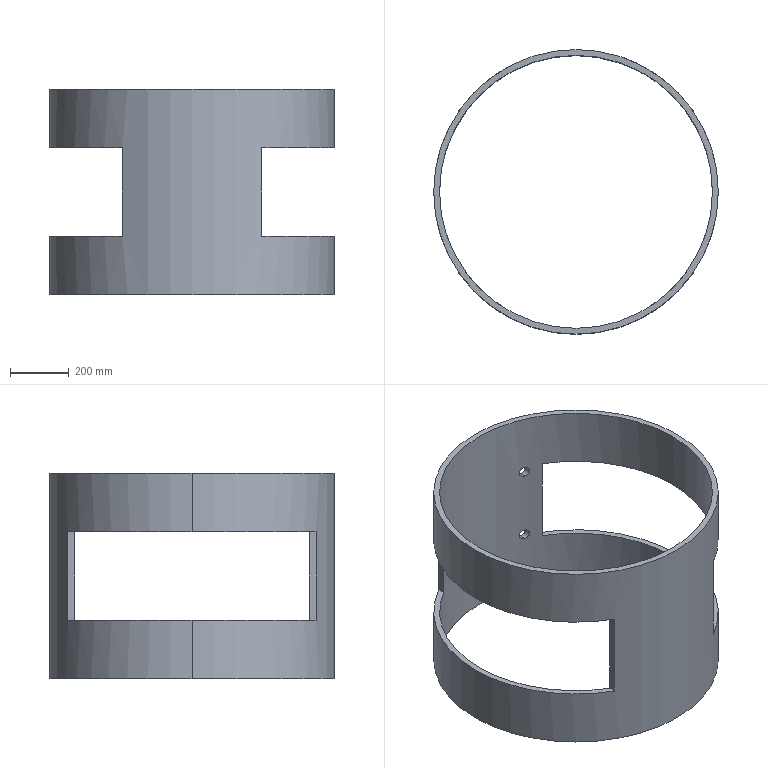Part | SolidWorks | features ICE 2, Extrusion 1 | 1 solid | 18 faces | box 970 x 970 x 700 mm | volume 29802772 mm3 | plane 10 | cylinder 8 | commonest cylinder face diameters 35 x4 930 x2 970 x2
STEP:
#1=CARTESIAN_POINT('',(180.,450.361,202.5));
#2=VERTEX_POINT('',#1);
#3=CARTESIAN_POINT('',(180.,450.361,237.5));
#4=VERTEX_POINT('',#3);
#5=CARTESIAN_POINT('',(180.,450.361,202.5));
#6=CARTESIAN_POINT('',(178.89,450.805,202.5));
#7=CARTESIAN_POINT('',(177.794,451.238,202.605));
#8=CARTESIAN_POINT('',(176.172,451.872,202.915));
#9=CARTESIAN_POINT('',(175.635,452.081,203.044));
#10=CARTESIAN_POINT('',(174.569,452.494,203.355));
#11=CARTESIAN_POINT('',(174.037,452.699,203.538));
#12=CARTESIAN_POINT('',(172.473,453.298,204.162));
#13=CARTESIAN_POINT('',(171.479,453.675,204.674));
#14=CARTESIAN_POINT('',(170.061,454.208,205.585));
#15=CARTESIAN_POINT('',(169.601,454.38,205.914));
#16=CARTESIAN_POINT('',(168.706,454.713,206.62));
#17=CARTESIAN_POINT('',(168.27,454.874,207.001));
#18=CARTESIAN_POINT('',(167.03,455.332,208.196));
#19=CARTESIAN_POINT('',(166.286,455.604,209.068));
#20=CARTESIAN_POINT('',(165.296,455.963,210.493));
#21=CARTESIAN_POINT('',(164.988,456.075,210.987));
#22=CARTESIAN_POINT('',(164.416,456.281,212.016));
#23=CARTESIAN_POINT('',(164.156,456.375,212.545));
#24=CARTESIAN_POINT('',(163.462,456.624,214.16));
#25=CARTESIAN_POINT('',(163.108,456.75,215.277));
#26=CARTESIAN_POINT('',(162.746,456.879,217.019));
#27=CARTESIAN_POINT('',(162.653,456.912,217.612));
#28=CARTESIAN_POINT('',(162.532,456.956,218.794));
#29=CARTESIAN_POINT('',(162.47,456.977,219.975));
#30=CARTESIAN_POINT('',(162.528,456.957,221.155));
#31=CARTESIAN_POINT('',(162.646,456.915,222.335));
#32=CARTESIAN_POINT('',(162.737,456.883,222.928));
#33=CARTESIAN_POINT('',(163.094,456.755,224.675));
#34=CARTESIAN_POINT('',(163.446,456.63,225.796));
#35=CARTESIAN_POINT('',(164.138,456.381,227.416));
#36=CARTESIAN_POINT('',(164.398,456.288,227.948));
#37=CARTESIAN_POINT('',(164.966,456.082,228.977));
#38=CARTESIAN_POINT('',(165.274,455.971,229.472));
#39=CARTESIAN_POINT('',(166.262,455.612,230.902));
#40=CARTESIAN_POINT('',(167.008,455.339,231.781));
#41=CARTESIAN_POINT('',(168.672,454.726,233.389));
#42=CARTESIAN_POINT('',(169.564,454.394,234.093));
#43=CARTESIAN_POINT('',(170.986,453.86,235.01));
#44=CARTESIAN_POINT('',(171.474,453.676,235.293));
#45=CARTESIAN_POINT('',(172.477,453.296,235.811));
#46=CARTESIAN_POINT('',(172.993,453.099,236.046));
#47=CARTESIAN_POINT('',(174.55,452.502,236.667));
#48=CARTESIAN_POINT('',(175.613,452.091,236.977));
#49=CARTESIAN_POINT('',(177.244,451.453,237.29));
#50=CARTESIAN_POINT('',(177.795,451.236,237.369));
#51=CARTESIAN_POINT('',(178.9,450.799,237.474));
#52=CARTESIAN_POINT('',(179.451,450.58,237.5));
#53=CARTESIAN_POINT('',(180.,450.361,237.5));
#54=B_SPLINE_CURVE_WITH_KNOTS('',3,(#5,#6,#7,#8,#9,#10,#11,#12,#13,#14,#15,#16,#17,#18,#19,#20,#21,#22,#23,#24,#25,#26,#27,#28,#29,#30,#31,#32,#33,#34,#35,#36,#37,#38,#39,#40,#41,#42,#43,#44,#45,#46,#47,#48,#49,#50,#51,#52,#53),.UNSPECIFIED.,.F.,.F.,(4,2,2,2,2,2,2,2,2,2,2,2,1,2,2,2,2,2,2,2,2,2,2,2,4),(0.,0.003538,0.005306,0.007075,0.01061,0.01238,0.01415,0.01769,0.01946,0.02123,0.02476,0.02653,0.0283,0.03007,0.03184,0.03538,0.03714,0.03891,0.04245,0.04599,0.04776,0.04953,0.05306,0.05483,0.0566),.UNSPECIFIED.);
#55=EDGE_CURVE('',#2,#4,#54,.T.);
#56=ORIENTED_EDGE('',*,*,#55,.T.);
#57=CARTESIAN_POINT('',(180.,428.748,237.5));
#58=VERTEX_POINT('',#57);
#59=CARTESIAN_POINT('',(180.,700.,237.5));
#60=DIRECTION('',(0.,-1.,0.));
#61=VECTOR('',#60,1000.);
#62=LINE('',#59,#61);
#63=EDGE_CURVE('',#4,#58,#62,.T.);
#64=ORIENTED_EDGE('',*,*,#63,.T.);
#65=CARTESIAN_POINT('',(180.,428.748,202.5));
#66=VERTEX_POINT('',#65);
#67=CARTESIAN_POINT('',(180.,428.748,202.5));
#68=CARTESIAN_POINT('',(178.894,429.213,202.5));
#69=CARTESIAN_POINT('',(177.802,429.666,202.604));
#70=CARTESIAN_POINT('',(176.186,430.33,202.912));
#71=CARTESIAN_POINT('',(175.65,430.549,203.04));
#72=CARTESIAN_POINT('',(174.587,430.981,203.349));
#73=CARTESIAN_POINT('',(174.057,431.196,203.531));
#74=CARTESIAN_POINT('',(172.495,431.824,204.151));
#75=CARTESIAN_POINT('',(171.502,432.219,204.661));
#76=CARTESIAN_POINT('',(170.085,432.778,205.569));
#77=CARTESIAN_POINT('',(169.625,432.958,205.896));
#78=CARTESIAN_POINT('',(168.73,433.307,206.6));
#79=CARTESIAN_POINT('',(168.294,433.477,206.979));
#80=CARTESIAN_POINT('',(167.05,433.958,208.173));
#81=CARTESIAN_POINT('',(166.304,434.245,209.045));
#82=CARTESIAN_POINT('',(165.312,434.623,210.468));
#83=CARTESIAN_POINT('',(165.003,434.74,210.962));
#84=CARTESIAN_POINT('',(164.573,434.903,211.733));
#85=CARTESIAN_POINT('',(164.435,434.955,211.996));
#86=CARTESIAN_POINT('',(164.174,435.054,212.525));
#87=CARTESIAN_POINT('',(164.051,435.1,212.792));
#88=CARTESIAN_POINT('',(163.468,435.32,214.14));
#89=CARTESIAN_POINT('',(163.112,435.453,215.261));
#90=CARTESIAN_POINT('',(162.748,435.589,217.005));
#91=CARTESIAN_POINT('',(162.655,435.624,217.601));
#92=CARTESIAN_POINT('',(162.532,435.67,218.787));
#93=CARTESIAN_POINT('',(162.501,435.682,219.38));
#94=CARTESIAN_POINT('',(162.499,435.682,220.565));
#95=CARTESIAN_POINT('',(162.528,435.671,221.157));
#96=CARTESIAN_POINT('',(162.617,435.638,222.044));
#97=CARTESIAN_POINT('',(162.655,435.624,222.34));
#98=CARTESIAN_POINT('',(162.745,435.591,222.931));
#99=CARTESIAN_POINT('',(162.798,435.571,223.227));
#100=CARTESIAN_POINT('',(163.098,435.459,224.688));
#101=CARTESIAN_POINT('',(163.452,435.326,225.813));
#102=CARTESIAN_POINT('',(164.147,435.064,227.435));
#103=CARTESIAN_POINT('',(164.408,434.966,227.967));
#104=CARTESIAN_POINT('',(164.979,434.749,228.998));
#105=CARTESIAN_POINT('',(165.288,434.632,229.494));
#106=CARTESIAN_POINT('',(166.279,434.254,230.924));
#107=CARTESIAN_POINT('',(167.028,433.967,231.803));
#108=CARTESIAN_POINT('',(168.694,433.322,233.407));
#109=CARTESIAN_POINT('',(169.587,432.974,234.11));
#110=CARTESIAN_POINT('',(171.008,432.414,235.024));
#111=CARTESIAN_POINT('',(171.496,432.22,235.305));
#112=CARTESIAN_POINT('',(172.498,431.821,235.821));
#113=CARTESIAN_POINT('',(173.013,431.615,236.054));
#114=CARTESIAN_POINT('',(174.567,430.99,236.673));
#115=CARTESIAN_POINT('',(175.628,430.559,236.981));
#116=CARTESIAN_POINT('',(177.253,429.891,237.292));
#117=CARTESIAN_POINT('',(177.803,429.664,237.37));
#118=CARTESIAN_POINT('',(178.904,429.207,237.474));
#119=CARTESIAN_POINT('',(179.453,428.978,237.5));
#120=CARTESIAN_POINT('',(180.,428.748,237.5));
#121=B_SPLINE_CURVE_WITH_KNOTS('',3,(#67,#68,#69,#70,#71,#72,#73,#74,#75,#76,#77,#78,#79,#80,#81,#82,#83,#84,#85,#86,#87,#88,#89,#90,#91,#92,#93,#94,#95,#96,#97,#98,#99,#100,#101,#102,#103,#104,#105,#106,#107,#108,#109,#110,#111,#112,#113,#114,#115,#116,#117,#118,#119,#120),.UNSPECIFIED.,.F.,.F.,(4,2,2,2,2,2,2,2,2,2,2,2,2,2,2,2,2,2,2,2,2,2,2,2,2,2,4),(0.,0.003549,0.005324,0.007098,0.01065,0.01242,0.0142,0.01775,0.01952,0.02041,0.0213,0.02484,0.02662,0.02839,0.03017,0.03106,0.03194,0.03549,0.03727,0.03904,0.04259,0.04614,0.04791,0.04969,0.05324,0.05501,0.05679),.UNSPECIFIED.);
#122=EDGE_CURVE('',#66,#58,#121,.T.);
#123=ORIENTED_EDGE('',*,*,#122,.F.);
#124=CARTESIAN_POINT('',(180.,700.,202.5));
#125=DIRECTION('',(0.,-1.,0.));
#126=VECTOR('',#125,1000.);
#127=LINE('',#124,#126);
#128=EDGE_CURVE('',#2,#66,#127,.T.);
#129=ORIENTED_EDGE('',*,*,#128,.F.);
#130=EDGE_LOOP('',(#56,#64,#123,#129));
#131=FACE_OUTER_BOUND('',#130,.T.);
#132=CARTESIAN_POINT('',(180.,700.,220.));
#133=DIRECTION('',(0.,-1.,0.));
#134=DIRECTION('',(0.,0.,-1.));
#135=AXIS2_PLACEMENT_3D('',#132,#133,#134);
#136=CYLINDRICAL_SURFACE('',#135,17.5);
#137=ADVANCED_FACE('',(#131),#136,.F.);
#138=CARTESIAN_POINT('',(180.,450.361,462.5));
#139=VERTEX_POINT('',#138);
#140=CARTESIAN_POINT('',(180.,450.361,497.5));
#141=VERTEX_POINT('',#140);
#142=CARTESIAN_POINT('',(180.,450.361,462.5));
#143=CARTESIAN_POINT('',(178.89,450.805,462.5));
#144=CARTESIAN_POINT('',(177.794,451.238,462.605));
#145=CARTESIAN_POINT('',(176.172,451.872,462.915));
#146=CARTESIAN_POINT('',(175.635,452.081,463.044));
#147=CARTESIAN_POINT('',(174.569,452.494,463.355));
#148=CARTESIAN_POINT('',(174.037,452.699,463.538));
#149=CARTESIAN_POINT('',(172.473,453.298,464.162));
#150=CARTESIAN_POINT('',(171.479,453.675,464.674));
#151=CARTESIAN_POINT('',(170.061,454.208,465.585));
#152=CARTESIAN_POINT('',(169.601,454.38,465.914));
#153=CARTESIAN_POINT('',(168.706,454.713,466.62));
#154=CARTESIAN_POINT('',(168.27,454.874,467.001));
#155=CARTESIAN_POINT('',(167.03,455.332,468.196));
#156=CARTESIAN_POINT('',(166.286,455.604,469.068));
#157=CARTESIAN_POINT('',(165.296,455.963,470.493));
#158=CARTESIAN_POINT('',(164.988,456.075,470.987));
#159=CARTESIAN_POINT('',(164.416,456.281,472.016));
#160=CARTESIAN_POINT('',(164.156,456.375,472.545));
#161=CARTESIAN_POINT('',(163.462,456.624,474.16));
#162=CARTESIAN_POINT('',(163.108,456.75,475.277));
#163=CARTESIAN_POINT('',(162.746,456.879,477.019));
#164=CARTESIAN_POINT('',(162.653,456.912,477.612));
#165=CARTESIAN_POINT('',(162.532,456.956,478.794));
#166=CARTESIAN_POINT('',(162.47,456.977,479.975));
#167=CARTESIAN_POINT('',(162.528,456.957,481.155));
#168=CARTESIAN_POINT('',(162.646,456.915,482.335));
#169=CARTESIAN_POINT('',(162.737,456.883,482.928));
#170=CARTESIAN_POINT('',(163.094,456.755,484.675));
#171=CARTESIAN_POINT('',(163.446,456.63,485.796));
#172=CARTESIAN_POINT('',(164.138,456.381,487.416));
#173=CARTESIAN_POINT('',(164.398,456.288,487.948));
#174=CARTESIAN_POINT('',(164.966,456.082,488.977));
#175=CARTESIAN_POINT('',(165.274,455.971,489.472));
#176=CARTESIAN_POINT('',(166.262,455.612,490.902));
#177=CARTESIAN_POINT('',(167.008,455.339,491.781));
#178=CARTESIAN_POINT('',(168.672,454.726,493.389));
#179=CARTESIAN_POINT('',(169.564,454.394,494.093));
#180=CARTESIAN_POINT('',(170.986,453.86,495.01));
#181=CARTESIAN_POINT('',(171.474,453.676,495.293));
#182=CARTESIAN_POINT('',(172.477,453.296,495.811));
#183=CARTESIAN_POINT('',(172.993,453.099,496.046));
#184=CARTESIAN_POINT('',(174.55,452.502,496.667));
#185=CARTESIAN_POINT('',(175.613,452.091,496.977));
#186=CARTESIAN_POINT('',(177.244,451.453,497.29));
#187=CARTESIAN_POINT('',(177.795,451.236,497.369));
#188=CARTESIAN_POINT('',(178.9,450.799,497.474));
#189=CARTESIAN_POINT('',(179.451,450.58,497.5));
#190=CARTESIAN_POINT('',(180.,450.361,497.5));
#191=B_SPLINE_CURVE_WITH_KNOTS('',3,(#142,#143,#144,#145,#146,#147,#148,#149,#150,#151,#152,#153,#154,#155,#156,#157,#158,#159,#160,#161,#162,#163,#164,#165,#166,#167,#168,#169,#170,#171,#172,#173,#174,#175,#176,#177,#178,#179,#180,#181,#182,#183,#184,#185,#186,#187,#188,#189,#190),.UNSPECIFIED.,.F.,.F.,(4,2,2,2,2,2,2,2,2,2,2,2,1,2,2,2,2,2,2,2,2,2,2,2,4),(0.,0.003538,0.005306,0.007075,0.01061,0.01238,0.01415,0.01769,0.01946,0.02123,0.02476,0.02653,0.0283,0.03007,0.03184,0.03538,0.03714,0.03891,0.04245,0.04599,0.04776,0.04953,0.05306,0.05483,0.0566),.UNSPECIFIED.);
#192=EDGE_CURVE('',#139,#141,#191,.T.);
#193=ORIENTED_EDGE('',*,*,#192,.T.);
#194=CARTESIAN_POINT('',(180.,428.748,497.5));
#195=VERTEX_POINT('',#194);
#196=CARTESIAN_POINT('',(180.,700.,497.5));
#197=DIRECTION('',(0.,-1.,0.));
#198=VECTOR('',#197,1000.);
#199=LINE('',#196,#198);
#200=EDGE_CURVE('',#141,#195,#199,.T.);
#201=ORIENTED_EDGE('',*,*,#200,.T.);
#202=CARTESIAN_POINT('',(180.,428.748,462.5));
#203=VERTEX_POINT('',#202);
#204=CARTESIAN_POINT('',(180.,428.748,462.5));
#205=CARTESIAN_POINT('',(178.894,429.213,462.5));
#206=CARTESIAN_POINT('',(177.802,429.666,462.604));
#207=CARTESIAN_POINT('',(176.186,430.33,462.912));
#208=CARTESIAN_POINT('',(175.65,430.549,463.04));
#209=CARTESIAN_POINT('',(174.587,430.981,463.349));
#210=CARTESIAN_POINT('',(174.057,431.196,463.531));
#211=CARTESIAN_POINT('',(172.495,431.824,464.151));
#212=CARTESIAN_POINT('',(171.502,432.219,464.661));
#213=CARTESIAN_POINT('',(170.085,432.778,465.569));
#214=CARTESIAN_POINT('',(169.625,432.958,465.896));
#215=CARTESIAN_POINT('',(168.73,433.307,466.6));
#216=CARTESIAN_POINT('',(168.294,433.477,466.979));
#217=CARTESIAN_POINT('',(167.05,433.958,468.173));
#218=CARTESIAN_POINT('',(166.304,434.245,469.045));
#219=CARTESIAN_POINT('',(165.312,434.623,470.468));
#220=CARTESIAN_POINT('',(165.003,434.74,470.962));
#221=CARTESIAN_POINT('',(164.573,434.903,471.733));
#222=CARTESIAN_POINT('',(164.435,434.955,471.996));
#223=CARTESIAN_POINT('',(164.174,435.054,472.525));
#224=CARTESIAN_POINT('',(164.051,435.1,472.792));
#225=CARTESIAN_POINT('',(163.468,435.32,474.14));
#226=CARTESIAN_POINT('',(163.112,435.453,475.261));
#227=CARTESIAN_POINT('',(162.748,435.589,477.005));
#228=CARTESIAN_POINT('',(162.655,435.624,477.601));
#229=CARTESIAN_POINT('',(162.532,435.67,478.787));
#230=CARTESIAN_POINT('',(162.501,435.682,479.38));
#231=CARTESIAN_POINT('',(162.499,435.682,480.565));
#232=CARTESIAN_POINT('',(162.528,435.671,481.157));
#233=CARTESIAN_POINT('',(162.617,435.638,482.044));
#234=CARTESIAN_POINT('',(162.655,435.624,482.34));
#235=CARTESIAN_POINT('',(162.745,435.591,482.931));
#236=CARTESIAN_POINT('',(162.798,435.571,483.227));
#237=CARTESIAN_POINT('',(163.098,435.459,484.688));
#238=CARTESIAN_POINT('',(163.452,435.326,485.813));
#239=CARTESIAN_POINT('',(164.147,435.064,487.435));
#240=CARTESIAN_POINT('',(164.408,434.966,487.967));
#241=CARTESIAN_POINT('',(164.979,434.749,488.998));
#242=CARTESIAN_POINT('',(165.288,434.632,489.494));
#243=CARTESIAN_POINT('',(166.279,434.254,490.924));
#244=CARTESIAN_POINT('',(167.028,433.967,491.803));
#245=CARTESIAN_POINT('',(168.694,433.322,493.407));
#246=CARTESIAN_POINT('',(169.587,432.974,494.11));
#247=CARTESIAN_POINT('',(171.008,432.414,495.024));
#248=CARTESIAN_POINT('',(171.496,432.22,495.305));
#249=CARTESIAN_POINT('',(172.498,431.821,495.821));
#250=CARTESIAN_POINT('',(173.013,431.615,496.054));
#251=CARTESIAN_POINT('',(174.567,430.99,496.673));
#252=CARTESIAN_POINT('',(175.628,430.559,496.981));
#253=CARTESIAN_POINT('',(177.253,429.891,497.292));
#254=CARTESIAN_POINT('',(177.803,429.664,497.37));
#255=CARTESIAN_POINT('',(178.904,429.207,497.474));
#256=CARTESIAN_POINT('',(179.453,428.978,497.5));
#257=CARTESIAN_POINT('',(180.,428.748,497.5));
#258=B_SPLINE_CURVE_WITH_KNOTS('',3,(#204,#205,#206,#207,#208,#209,#210,#211,#212,#213,#214,#215,#216,#217,#218,#219,#220,#221,#222,#223,#224,#225,#226,#227,#228,#229,#230,#231,#232,#233,#234,#235,#236,#237,#238,#239,#240,#241,#242,#243,#244,#245,#246,#247,#248,#249,#250,#251,#252,#253,#254,#255,#256,#257),.UNSPECIFIED.,.F.,.F.,(4,2,2,2,2,2,2,2,2,2,2,2,2,2,2,2,2,2,2,2,2,2,2,2,2,2,4),(0.,0.003549,0.005324,0.007098,0.01065,0.01242,0.0142,0.01775,0.01952,0.02041,0.0213,0.02484,0.02662,0.02839,0.03017,0.03106,0.03194,0.03549,0.03727,0.03904,0.04259,0.04614,0.04791,0.04969,0.05324,0.05501,0.05679),.UNSPECIFIED.);
#259=EDGE_CURVE('',#203,#195,#258,.T.);
#260=ORIENTED_EDGE('',*,*,#259,.F.);
#261=CARTESIAN_POINT('',(180.,700.,462.5));
#262=DIRECTION('',(0.,-1.,0.));
#263=VECTOR('',#262,1000.);
#264=LINE('',#261,#263);
#265=EDGE_CURVE('',#139,#203,#264,.T.);
#266=ORIENTED_EDGE('',*,*,#265,.F.);
#267=EDGE_LOOP('',(#193,#201,#260,#266));
#268=FACE_OUTER_BOUND('',#267,.T.);
#269=CARTESIAN_POINT('',(180.,700.,480.));
#270=DIRECTION('',(0.,-1.,0.));
#271=DIRECTION('',(0.,0.,-1.));
#272=AXIS2_PLACEMENT_3D('',#269,#270,#271);
#273=CYLINDRICAL_SURFACE('',#272,17.5);
#274=ADVANCED_FACE('',(#268),#273,.F.);
#275=CARTESIAN_POINT('',(-465.,0.,700.));
#276=VERTEX_POINT('',#275);
#277=CARTESIAN_POINT('',(465.,0.,700.));
#278=VERTEX_POINT('',#277);
#279=CARTESIAN_POINT('',(0.,0.,700.));
#280=DIRECTION('',(0.,0.,1.));
#281=DIRECTION('',(1.,0.,0.));
#282=AXIS2_PLACEMENT_3D('',#279,#280,#281);
#283=CIRCLE('',#282,465.);
#284=EDGE_CURVE('',#276,#278,#283,.T.);
#285=ORIENTED_EDGE('',*,*,#284,.T.);
#286=CARTESIAN_POINT('',(465.,0.,500.));
#287=VERTEX_POINT('',#286);
#288=CARTESIAN_POINT('',(465.,0.,700.));
#289=DIRECTION('',(0.,0.,-1.));
#290=VECTOR('',#289,1000.);
#291=LINE('',#288,#290);
#292=EDGE_CURVE('',#278,#287,#291,.T.);
#293=ORIENTED_EDGE('',*,*,#292,.T.);
#294=CARTESIAN_POINT('',(237.5,-399.773,500.));
#295=VERTEX_POINT('',#294);
#296=CARTESIAN_POINT('',(0.,0.,500.));
#297=DIRECTION('',(0.,0.,1.));
#298=DIRECTION('',(1.,0.,0.));
#299=AXIS2_PLACEMENT_3D('',#296,#297,#298);
#300=CIRCLE('',#299,465.);
#301=EDGE_CURVE('',#295,#287,#300,.T.);
#302=ORIENTED_EDGE('',*,*,#301,.F.);
#303=CARTESIAN_POINT('',(237.5,-399.773,200.));
#304=VERTEX_POINT('',#303);
#305=CARTESIAN_POINT('',(237.5,-399.773,700.));
#306=DIRECTION('',(0.,0.,1.));
#307=VECTOR('',#306,1000.);
#308=LINE('',#305,#307);
#309=EDGE_CURVE('',#304,#295,#308,.T.);
#310=ORIENTED_EDGE('',*,*,#309,.F.);
#311=CARTESIAN_POINT('',(465.,0.,200.));
#312=VERTEX_POINT('',#311);
#313=CARTESIAN_POINT('',(0.,0.,200.));
#314=DIRECTION('',(0.,0.,-1.));
#315=DIRECTION('',(-1.,0.,0.));
#316=AXIS2_PLACEMENT_3D('',#313,#314,#315);
#317=CIRCLE('',#316,465.);
#318=EDGE_CURVE('',#312,#304,#317,.T.);
#319=ORIENTED_EDGE('',*,*,#318,.F.);
#320=CARTESIAN_POINT('',(465.,0.,0.));
#321=VERTEX_POINT('',#320);
#322=CARTESIAN_POINT('',(465.,0.,700.));
#323=DIRECTION('',(0.,0.,-1.));
#324=VECTOR('',#323,1000.);
#325=LINE('',#322,#324);
#326=EDGE_CURVE('',#312,#321,#325,.T.);
#327=ORIENTED_EDGE('',*,*,#326,.T.);
#328=CARTESIAN_POINT('',(-465.,0.,0.));
#329=VERTEX_POINT('',#328);
#330=CARTESIAN_POINT('',(0.,0.,0.));
#331=DIRECTION('',(0.,0.,1.));
#332=DIRECTION('',(1.,0.,0.));
#333=AXIS2_PLACEMENT_3D('',#330,#331,#332);
#334=CIRCLE('',#333,465.);
#335=EDGE_CURVE('',#329,#321,#334,.T.);
#336=ORIENTED_EDGE('',*,*,#335,.F.);
#337=CARTESIAN_POINT('',(-465.,0.,200.));
#338=VERTEX_POINT('',#337);
#339=CARTESIAN_POINT('',(-465.,0.,700.));
#340=DIRECTION('',(0.,0.,-1.));
#341=VECTOR('',#340,1000.);
#342=LINE('',#339,#341);
#343=EDGE_CURVE('',#338,#329,#342,.T.);
#344=ORIENTED_EDGE('',*,*,#343,.F.);
#345=CARTESIAN_POINT('',(-237.5,-399.773,200.));
#346=VERTEX_POINT('',#345);
#347=CARTESIAN_POINT('',(0.,0.,200.));
#348=DIRECTION('',(0.,0.,-1.));
#349=DIRECTION('',(-1.,0.,0.));
#350=AXIS2_PLACEMENT_3D('',#347,#348,#349);
#351=CIRCLE('',#350,465.);
#352=EDGE_CURVE('',#346,#338,#351,.T.);
#353=ORIENTED_EDGE('',*,*,#352,.F.);
#354=CARTESIAN_POINT('',(-237.5,-399.773,500.));
#355=VERTEX_POINT('',#354);
#356=CARTESIAN_POINT('',(-237.5,-399.773,700.));
#357=DIRECTION('',(0.,0.,-1.));
#358=VECTOR('',#357,1000.);
#359=LINE('',#356,#358);
#360=EDGE_CURVE('',#355,#346,#359,.T.);
#361=ORIENTED_EDGE('',*,*,#360,.F.);
#362=CARTESIAN_POINT('',(-465.,0.,500.));
#363=VERTEX_POINT('',#362);
#364=CARTESIAN_POINT('',(0.,0.,500.));
#365=DIRECTION('',(0.,0.,1.));
#366=DIRECTION('',(1.,0.,0.));
#367=AXIS2_PLACEMENT_3D('',#364,#365,#366);
#368=CIRCLE('',#367,465.);
#369=EDGE_CURVE('',#363,#355,#368,.T.);
#370=ORIENTED_EDGE('',*,*,#369,.F.);
#371=CARTESIAN_POINT('',(-465.,0.,700.));
#372=DIRECTION('',(0.,0.,-1.));
#373=VECTOR('',#372,1000.);
#374=LINE('',#371,#373);
#375=EDGE_CURVE('',#276,#363,#374,.T.);
#376=ORIENTED_EDGE('',*,*,#375,.F.);
#377=EDGE_LOOP('',(#285,#293,#302,#310,#319,#327,#336,#344,#353,#361,#370,#376));
#378=FACE_OUTER_BOUND('',#377,.T.);
#379=CARTESIAN_POINT('',(0.,0.,700.));
#380=DIRECTION('',(0.,0.,-1.));
#381=DIRECTION('',(-1.,0.,0.));
#382=AXIS2_PLACEMENT_3D('',#379,#380,#381);
#383=CYLINDRICAL_SURFACE('',#382,465.);
#384=ADVANCED_FACE('',(#378),#383,.F.);
#385=ORIENTED_EDGE('',*,*,#192,.F.);
#386=CARTESIAN_POINT('',(180.,450.361,497.5));
#387=CARTESIAN_POINT('',(181.105,449.919,497.5));
#388=CARTESIAN_POINT('',(182.202,449.476,497.396));
#389=CARTESIAN_POINT('',(183.837,448.809,497.083));
#390=CARTESIAN_POINT('',(184.383,448.585,496.951));
#391=CARTESIAN_POINT('',(185.45,448.144,496.639));
#392=CARTESIAN_POINT('',(185.974,447.927,496.458));
#393=CARTESIAN_POINT('',(187.517,447.285,495.842));
#394=CARTESIAN_POINT('',(188.507,446.868,495.335));
#395=CARTESIAN_POINT('',(189.931,446.264,494.42));
#396=CARTESIAN_POINT('',(190.395,446.066,494.089));
#397=CARTESIAN_POINT('',(191.284,445.686,493.388));
#398=CARTESIAN_POINT('',(191.71,445.503,493.017));
#399=CARTESIAN_POINT('',(192.935,444.974,491.841));
#400=CARTESIAN_POINT('',(193.68,444.65,490.975));
#401=CARTESIAN_POINT('',(194.683,444.211,489.54));
#402=CARTESIAN_POINT('',(194.993,444.075,489.044));
#403=CARTESIAN_POINT('',(195.561,443.825,488.028));
#404=CARTESIAN_POINT('',(195.819,443.711,487.506));
#405=CARTESIAN_POINT('',(196.285,443.506,486.435));
#406=CARTESIAN_POINT('',(196.491,443.414,485.885));
#407=CARTESIAN_POINT('',(196.851,443.255,484.758));
#408=CARTESIAN_POINT('',(197.005,443.186,484.176));
#409=CARTESIAN_POINT('',(197.372,443.023,482.423));
#410=CARTESIAN_POINT('',(197.496,442.967,481.243));
#411=CARTESIAN_POINT('',(197.501,442.966,479.752));
#412=CARTESIAN_POINT('',(197.494,442.969,479.453));
#413=CARTESIAN_POINT('',(197.465,442.981,478.854));
#414=CARTESIAN_POINT('',(197.443,442.991,478.553));
#415=CARTESIAN_POINT('',(197.353,443.031,477.656));
#416=CARTESIAN_POINT('',(197.263,443.072,477.067));
#417=CARTESIAN_POINT('',(197.024,443.178,475.905));
#418=CARTESIAN_POINT('',(196.876,443.243,475.332));
#419=CARTESIAN_POINT('',(196.523,443.4,474.203));
#420=CARTESIAN_POINT('',(196.316,443.492,473.644));
#421=CARTESIAN_POINT('',(195.615,443.802,472.011));
#422=CARTESIAN_POINT('',(195.048,444.051,470.992));
#423=CARTESIAN_POINT('',(194.06,444.484,469.564));
#424=CARTESIAN_POINT('',(193.705,444.639,469.103));
#425=CARTESIAN_POINT('',(192.955,444.965,468.22));
#426=CARTESIAN_POINT('',(192.562,445.135,467.803));
#427=CARTESIAN_POINT('',(191.333,445.665,466.617));
#428=CARTESIAN_POINT('',(190.447,446.045,465.915));
#429=CARTESIAN_POINT('',(189.02,446.651,464.993));
#430=CARTESIAN_POINT('',(188.531,446.857,464.71));
#431=CARTESIAN_POINT('',(187.538,447.275,464.197));
#432=CARTESIAN_POINT('',(187.032,447.487,463.965));
#433=CARTESIAN_POINT('',(186.002,447.916,463.552));
#434=CARTESIAN_POINT('',(185.478,448.133,463.37));
#435=CARTESIAN_POINT('',(184.412,448.573,463.056));
#436=CARTESIAN_POINT('',(183.867,448.796,462.924));
#437=CARTESIAN_POINT('',(182.225,449.467,462.606));
#438=CARTESIAN_POINT('',(181.117,449.914,462.5));
#439=CARTESIAN_POINT('',(180.,450.361,462.5));
#440=B_SPLINE_CURVE_WITH_KNOTS('',3,(#386,#387,#388,#389,#390,#391,#392,#393,#394,#395,#396,#397,#398,#399,#400,#401,#402,#403,#404,#405,#406,#407,#408,#409,#410,#411,#412,#413,#414,#415,#416,#417,#418,#419,#420,#421,#422,#423,#424,#425,#426,#427,#428,#429,#430,#431,#432,#433,#434,#435,#436,#437,#438,#439),.UNSPECIFIED.,.F.,.F.,(4,2,2,2,2,2,2,2,2,2,2,2,2,2,2,2,2,2,2,2,2,2,2,2,2,2,4),(0.0566,0.06016,0.06194,0.06372,0.06728,0.06906,0.07084,0.0744,0.07618,0.07796,0.07974,0.08152,0.08508,0.08597,0.08686,0.08865,0.09043,0.09221,0.09577,0.09755,0.09933,0.1029,0.1047,0.1064,0.1082,0.11,0.1136),.UNSPECIFIED.);
#441=EDGE_CURVE('',#141,#139,#440,.T.);
#442=ORIENTED_EDGE('',*,*,#441,.F.);
#443=EDGE_LOOP('',(#385,#442));
#444=FACE_BOUND('',#443,.T.);
#445=ORIENTED_EDGE('',*,*,#55,.F.);
#446=CARTESIAN_POINT('',(180.,450.361,237.5));
#447=CARTESIAN_POINT('',(181.105,449.919,237.5));
#448=CARTESIAN_POINT('',(182.202,449.476,237.396));
#449=CARTESIAN_POINT('',(183.837,448.809,237.083));
#450=CARTESIAN_POINT('',(184.383,448.585,236.951));
#451=CARTESIAN_POINT('',(185.45,448.144,236.639));
#452=CARTESIAN_POINT('',(185.974,447.927,236.458));
#453=CARTESIAN_POINT('',(187.517,447.285,235.842));
#454=CARTESIAN_POINT('',(188.507,446.868,235.335));
#455=CARTESIAN_POINT('',(189.931,446.264,234.42));
#456=CARTESIAN_POINT('',(190.395,446.066,234.089));
#457=CARTESIAN_POINT('',(191.284,445.686,233.388));
#458=CARTESIAN_POINT('',(191.71,445.503,233.017));
#459=CARTESIAN_POINT('',(192.935,444.974,231.841));
#460=CARTESIAN_POINT('',(193.68,444.65,230.975));
#461=CARTESIAN_POINT('',(194.683,444.211,229.54));
#462=CARTESIAN_POINT('',(194.993,444.075,229.044));
#463=CARTESIAN_POINT('',(195.561,443.825,228.028));
#464=CARTESIAN_POINT('',(195.819,443.711,227.506));
#465=CARTESIAN_POINT('',(196.285,443.506,226.435));
#466=CARTESIAN_POINT('',(196.491,443.414,225.885));
#467=CARTESIAN_POINT('',(196.851,443.255,224.758));
#468=CARTESIAN_POINT('',(197.005,443.186,224.176));
#469=CARTESIAN_POINT('',(197.372,443.023,222.423));
#470=CARTESIAN_POINT('',(197.496,442.967,221.243));
#471=CARTESIAN_POINT('',(197.501,442.966,219.752));
#472=CARTESIAN_POINT('',(197.494,442.969,219.453));
#473=CARTESIAN_POINT('',(197.465,442.981,218.854));
#474=CARTESIAN_POINT('',(197.443,442.991,218.553));
#475=CARTESIAN_POINT('',(197.353,443.031,217.656));
#476=CARTESIAN_POINT('',(197.263,443.072,217.067));
#477=CARTESIAN_POINT('',(197.024,443.178,215.905));
#478=CARTESIAN_POINT('',(196.876,443.243,215.332));
#479=CARTESIAN_POINT('',(196.523,443.4,214.203));
#480=CARTESIAN_POINT('',(196.316,443.492,213.644));
#481=CARTESIAN_POINT('',(195.615,443.802,212.011));
#482=CARTESIAN_POINT('',(195.048,444.051,210.992));
#483=CARTESIAN_POINT('',(194.06,444.484,209.564));
#484=CARTESIAN_POINT('',(193.705,444.639,209.103));
#485=CARTESIAN_POINT('',(192.955,444.965,208.22));
#486=CARTESIAN_POINT('',(192.562,445.135,207.803));
#487=CARTESIAN_POINT('',(191.333,445.665,206.617));
#488=CARTESIAN_POINT('',(190.447,446.045,205.915));
#489=CARTESIAN_POINT('',(189.02,446.651,204.993));
#490=CARTESIAN_POINT('',(188.531,446.857,204.71));
#491=CARTESIAN_POINT('',(187.538,447.275,204.197));
#492=CARTESIAN_POINT('',(187.032,447.487,203.965));
#493=CARTESIAN_POINT('',(186.002,447.916,203.552));
#494=CARTESIAN_POINT('',(185.478,448.133,203.37));
#495=CARTESIAN_POINT('',(184.412,448.573,203.056));
#496=CARTESIAN_POINT('',(183.867,448.796,202.924));
#497=CARTESIAN_POINT('',(182.225,449.467,202.606));
#498=CARTESIAN_POINT('',(181.117,449.914,202.5));
#499=CARTESIAN_POINT('',(180.,450.361,202.5));
#500=B_SPLINE_CURVE_WITH_KNOTS('',3,(#446,#447,#448,#449,#450,#451,#452,#453,#454,#455,#456,#457,#458,#459,#460,#461,#462,#463,#464,#465,#466,#467,#468,#469,#470,#471,#472,#473,#474,#475,#476,#477,#478,#479,#480,#481,#482,#483,#484,#485,#486,#487,#488,#489,#490,#491,#492,#493,#494,#495,#496,#497,#498,#499),.UNSPECIFIED.,.F.,.F.,(4,2,2,2,2,2,2,2,2,2,2,2,2,2,2,2,2,2,2,2,2,2,2,2,2,2,4),(0.0566,0.06016,0.06194,0.06372,0.06728,0.06906,0.07084,0.0744,0.07618,0.07796,0.07974,0.08152,0.08508,0.08597,0.08686,0.08865,0.09043,0.09221,0.09577,0.09755,0.09933,0.1029,0.1047,0.1064,0.1082,0.11,0.1136),.UNSPECIFIED.);
#501=EDGE_CURVE('',#4,#2,#500,.T.);
#502=ORIENTED_EDGE('',*,*,#501,.F.);
#503=EDGE_LOOP('',(#445,#502));
#504=FACE_BOUND('',#503,.T.);
#505=CARTESIAN_POINT('',(485.,0.,700.));
#506=VERTEX_POINT('',#505);
#507=CARTESIAN_POINT('',(-485.,0.,700.));
#508=VERTEX_POINT('',#507);
#509=CARTESIAN_POINT('',(0.,0.,700.));
#510=DIRECTION('',(0.,0.,1.));
#511=DIRECTION('',(1.,0.,0.));
#512=AXIS2_PLACEMENT_3D('',#509,#510,#511);
#513=CIRCLE('',#512,485.);
#514=EDGE_CURVE('',#506,#508,#513,.T.);
#515=ORIENTED_EDGE('',*,*,#514,.F.);
#516=CARTESIAN_POINT('',(485.,0.,500.));
#517=VERTEX_POINT('',#516);
#518=CARTESIAN_POINT('',(485.,0.,700.));
#519=DIRECTION('',(0.,0.,-1.));
#520=VECTOR('',#519,1000.);
#521=LINE('',#518,#520);
#522=EDGE_CURVE('',#506,#517,#521,.T.);
#523=ORIENTED_EDGE('',*,*,#522,.T.);
#524=CARTESIAN_POINT('',(237.5,422.87,500.));
#525=VERTEX_POINT('',#524);
#526=CARTESIAN_POINT('',(0.,0.,500.));
#527=DIRECTION('',(0.,0.,1.));
#528=DIRECTION('',(1.,0.,0.));
#529=AXIS2_PLACEMENT_3D('',#526,#527,#528);
#530=CIRCLE('',#529,485.);
#531=EDGE_CURVE('',#517,#525,#530,.T.);
#532=ORIENTED_EDGE('',*,*,#531,.T.);
#533=CARTESIAN_POINT('',(237.5,422.87,200.));
#534=VERTEX_POINT('',#533);
#535=CARTESIAN_POINT('',(237.5,422.87,700.));
#536=DIRECTION('',(0.,0.,-1.));
#537=VECTOR('',#536,1000.);
#538=LINE('',#535,#537);
#539=EDGE_CURVE('',#525,#534,#538,.T.);
#540=ORIENTED_EDGE('',*,*,#539,.T.);
#541=CARTESIAN_POINT('',(485.,0.,200.));
#542=VERTEX_POINT('',#541);
#543=CARTESIAN_POINT('',(0.,0.,200.));
#544=DIRECTION('',(0.,0.,-1.));
#545=DIRECTION('',(-1.,0.,0.));
#546=AXIS2_PLACEMENT_3D('',#543,#544,#545);
#547=CIRCLE('',#546,485.);
#548=EDGE_CURVE('',#534,#542,#547,.T.);
#549=ORIENTED_EDGE('',*,*,#548,.T.);
#550=CARTESIAN_POINT('',(485.,0.,0.));
#551=VERTEX_POINT('',#550);
#552=CARTESIAN_POINT('',(485.,0.,700.));
#553=DIRECTION('',(0.,0.,-1.));
#554=VECTOR('',#553,1000.);
#555=LINE('',#552,#554);
#556=EDGE_CURVE('',#542,#551,#555,.T.);
#557=ORIENTED_EDGE('',*,*,#556,.T.);
#558=CARTESIAN_POINT('',(-485.,0.,0.));
#559=VERTEX_POINT('',#558);
#560=CARTESIAN_POINT('',(0.,0.,0.));
#561=DIRECTION('',(0.,0.,1.));
#562=DIRECTION('',(1.,0.,0.));
#563=AXIS2_PLACEMENT_3D('',#560,#561,#562);
#564=CIRCLE('',#563,485.);
#565=EDGE_CURVE('',#551,#559,#564,.T.);
#566=ORIENTED_EDGE('',*,*,#565,.T.);
#567=CARTESIAN_POINT('',(-485.,0.,200.));
#568=VERTEX_POINT('',#567);
#569=CARTESIAN_POINT('',(-485.,0.,700.));
#570=DIRECTION('',(0.,0.,-1.));
#571=VECTOR('',#570,1000.);
#572=LINE('',#569,#571);
#573=EDGE_CURVE('',#568,#559,#572,.T.);
#574=ORIENTED_EDGE('',*,*,#573,.F.);
#575=CARTESIAN_POINT('',(-237.5,422.87,200.));
#576=VERTEX_POINT('',#575);
#577=CARTESIAN_POINT('',(0.,0.,200.));
#578=DIRECTION('',(0.,0.,-1.));
#579=DIRECTION('',(-1.,0.,0.));
#580=AXIS2_PLACEMENT_3D('',#577,#578,#579);
#581=CIRCLE('',#580,485.);
#582=EDGE_CURVE('',#568,#576,#581,.T.);
#583=ORIENTED_EDGE('',*,*,#582,.T.);
#584=CARTESIAN_POINT('',(-237.5,422.87,500.));
#585=VERTEX_POINT('',#584);
#586=CARTESIAN_POINT('',(-237.5,422.87,700.));
#587=DIRECTION('',(0.,0.,1.));
#588=VECTOR('',#587,1000.);
#589=LINE('',#586,#588);
#590=EDGE_CURVE('',#576,#585,#589,.T.);
#591=ORIENTED_EDGE('',*,*,#590,.T.);
#592=CARTESIAN_POINT('',(-485.,0.,500.));
#593=VERTEX_POINT('',#592);
#594=CARTESIAN_POINT('',(0.,0.,500.));
#595=DIRECTION('',(0.,0.,1.));
#596=DIRECTION('',(1.,0.,0.));
#597=AXIS2_PLACEMENT_3D('',#594,#595,#596);
#598=CIRCLE('',#597,485.);
#599=EDGE_CURVE('',#585,#593,#598,.T.);
#600=ORIENTED_EDGE('',*,*,#599,.T.);
#601=CARTESIAN_POINT('',(-485.,0.,700.));
#602=DIRECTION('',(0.,0.,-1.));
#603=VECTOR('',#602,1000.);
#604=LINE('',#601,#603);
#605=EDGE_CURVE('',#508,#593,#604,.T.);
#606=ORIENTED_EDGE('',*,*,#605,.F.);
#607=EDGE_LOOP('',(#515,#523,#532,#540,#549,#557,#566,#574,#583,#591,#600,#606));
#608=FACE_OUTER_BOUND('',#607,.T.);
#609=CARTESIAN_POINT('',(0.,0.,700.));
#610=DIRECTION('',(0.,0.,-1.));
#611=DIRECTION('',(-1.,0.,0.));
#612=AXIS2_PLACEMENT_3D('',#609,#610,#611);
#613=CYLINDRICAL_SURFACE('',#612,485.);
#614=ADVANCED_FACE('',(#444,#504,#608),#613,.T.);
#615=ORIENTED_EDGE('',*,*,#522,.F.);
#616=CARTESIAN_POINT('',(0.,0.,700.));
#617=DIRECTION('',(0.,0.,1.));
#618=DIRECTION('',(1.,0.,0.));
#619=AXIS2_PLACEMENT_3D('',#616,#617,#618);
#620=CIRCLE('',#619,485.);
#621=EDGE_CURVE('',#508,#506,#620,.T.);
#622=ORIENTED_EDGE('',*,*,#621,.F.);
#623=ORIENTED_EDGE('',*,*,#605,.T.);
#624=CARTESIAN_POINT('',(-237.5,-422.87,500.));
#625=VERTEX_POINT('',#624);
#626=CARTESIAN_POINT('',(0.,0.,500.));
#627=DIRECTION('',(0.,0.,1.));
#628=DIRECTION('',(1.,0.,0.));
#629=AXIS2_PLACEMENT_3D('',#626,#627,#628);
#630=CIRCLE('',#629,485.);
#631=EDGE_CURVE('',#593,#625,#630,.T.);
#632=ORIENTED_EDGE('',*,*,#631,.T.);
#633=CARTESIAN_POINT('',(-237.5,-422.87,200.));
#634=VERTEX_POINT('',#633);
#635=CARTESIAN_POINT('',(-237.5,-422.87,700.));
#636=DIRECTION('',(0.,0.,-1.));
#637=VECTOR('',#636,1000.);
#638=LINE('',#635,#637);
#639=EDGE_CURVE('',#625,#634,#638,.T.);
#640=ORIENTED_EDGE('',*,*,#639,.T.);
#641=CARTESIAN_POINT('',(0.,0.,200.));
#642=DIRECTION('',(0.,0.,-1.));
#643=DIRECTION('',(-1.,0.,0.));
#644=AXIS2_PLACEMENT_3D('',#641,#642,#643);
#645=CIRCLE('',#644,485.);
#646=EDGE_CURVE('',#634,#568,#645,.T.);
#647=ORIENTED_EDGE('',*,*,#646,.T.);
#648=ORIENTED_EDGE('',*,*,#573,.T.);
#649=CARTESIAN_POINT('',(0.,0.,0.));
#650=DIRECTION('',(0.,0.,1.));
#651=DIRECTION('',(1.,0.,0.));
#652=AXIS2_PLACEMENT_3D('',#649,#650,#651);
#653=CIRCLE('',#652,485.);
#654=EDGE_CURVE('',#559,#551,#653,.T.);
#655=ORIENTED_EDGE('',*,*,#654,.T.);
#656=ORIENTED_EDGE('',*,*,#556,.F.);
#657=CARTESIAN_POINT('',(237.5,-422.87,200.));
#658=VERTEX_POINT('',#657);
#659=CARTESIAN_POINT('',(0.,0.,200.));
#660=DIRECTION('',(0.,0.,-1.));
#661=DIRECTION('',(-1.,0.,0.));
#662=AXIS2_PLACEMENT_3D('',#659,#660,#661);
#663=CIRCLE('',#662,485.);
#664=EDGE_CURVE('',#542,#658,#663,.T.);
#665=ORIENTED_EDGE('',*,*,#664,.T.);
#666=CARTESIAN_POINT('',(237.5,-422.87,500.));
#667=VERTEX_POINT('',#666);
#668=CARTESIAN_POINT('',(237.5,-422.87,700.));
#669=DIRECTION('',(0.,0.,1.));
#670=VECTOR('',#669,1000.);
#671=LINE('',#668,#670);
#672=EDGE_CURVE('',#658,#667,#671,.T.);
#673=ORIENTED_EDGE('',*,*,#672,.T.);
#674=CARTESIAN_POINT('',(0.,0.,500.));
#675=DIRECTION('',(0.,0.,1.));
#676=DIRECTION('',(1.,0.,0.));
#677=AXIS2_PLACEMENT_3D('',#674,#675,#676);
#678=CIRCLE('',#677,485.);
#679=EDGE_CURVE('',#667,#517,#678,.T.);
#680=ORIENTED_EDGE('',*,*,#679,.T.);
#681=EDGE_LOOP('',(#615,#622,#623,#632,#640,#647,#648,#655,#656,#665,#673,#680));
#682=FACE_OUTER_BOUND('',#681,.T.);
#683=CARTESIAN_POINT('',(0.,0.,700.));
#684=DIRECTION('',(0.,0.,-1.));
#685=DIRECTION('',(-1.,0.,0.));
#686=AXIS2_PLACEMENT_3D('',#683,#684,#685);
#687=CYLINDRICAL_SURFACE('',#686,485.);
#688=ADVANCED_FACE('',(#682),#687,.T.);
#689=ORIENTED_EDGE('',*,*,#292,.F.);
#690=CARTESIAN_POINT('',(0.,0.,700.));
#691=DIRECTION('',(0.,0.,1.));
#692=DIRECTION('',(1.,0.,0.));
#693=AXIS2_PLACEMENT_3D('',#690,#691,#692);
#694=CIRCLE('',#693,465.);
#695=EDGE_CURVE('',#278,#276,#694,.T.);
#696=ORIENTED_EDGE('',*,*,#695,.T.);
#697=ORIENTED_EDGE('',*,*,#375,.T.);
#698=CARTESIAN_POINT('',(-237.5,399.773,500.));
#699=VERTEX_POINT('',#698);
#700=CARTESIAN_POINT('',(0.,0.,500.));
#701=DIRECTION('',(0.,0.,1.));
#702=DIRECTION('',(1.,0.,0.));
#703=AXIS2_PLACEMENT_3D('',#700,#701,#702);
#704=CIRCLE('',#703,465.);
#705=EDGE_CURVE('',#699,#363,#704,.T.);
#706=ORIENTED_EDGE('',*,*,#705,.F.);
#707=CARTESIAN_POINT('',(-237.5,399.773,200.));
#708=VERTEX_POINT('',#707);
#709=CARTESIAN_POINT('',(-237.5,399.773,700.));
#710=DIRECTION('',(0.,0.,1.));
#711=VECTOR('',#710,1000.);
#712=LINE('',#709,#711);
#713=EDGE_CURVE('',#708,#699,#712,.T.);
#714=ORIENTED_EDGE('',*,*,#713,.F.);
#715=CARTESIAN_POINT('',(0.,0.,200.));
#716=DIRECTION('',(0.,0.,-1.));
#717=DIRECTION('',(-1.,0.,0.));
#718=AXIS2_PLACEMENT_3D('',#715,#716,#717);
#719=CIRCLE('',#718,465.);
#720=EDGE_CURVE('',#338,#708,#719,.T.);
#721=ORIENTED_EDGE('',*,*,#720,.F.);
#722=ORIENTED_EDGE('',*,*,#343,.T.);
#723=CARTESIAN_POINT('',(0.,0.,0.));
#724=DIRECTION('',(0.,0.,1.));
#725=DIRECTION('',(1.,0.,0.));
#726=AXIS2_PLACEMENT_3D('',#723,#724,#725);
#727=CIRCLE('',#726,465.);
#728=EDGE_CURVE('',#321,#329,#727,.T.);
#729=ORIENTED_EDGE('',*,*,#728,.F.);
#730=ORIENTED_EDGE('',*,*,#326,.F.);
#731=CARTESIAN_POINT('',(237.5,399.773,200.));
#732=VERTEX_POINT('',#731);
#733=CARTESIAN_POINT('',(0.,0.,200.));
#734=DIRECTION('',(0.,0.,-1.));
#735=DIRECTION('',(-1.,0.,0.));
#736=AXIS2_PLACEMENT_3D('',#733,#734,#735);
#737=CIRCLE('',#736,465.);
#738=EDGE_CURVE('',#732,#312,#737,.T.);
#739=ORIENTED_EDGE('',*,*,#738,.F.);
#740=CARTESIAN_POINT('',(237.5,399.773,500.));
#741=VERTEX_POINT('',#740);
#742=CARTESIAN_POINT('',(237.5,399.773,700.));
#743=DIRECTION('',(0.,0.,-1.));
#744=VECTOR('',#743,1000.);
#745=LINE('',#742,#744);
#746=EDGE_CURVE('',#741,#732,#745,.T.);
#747=ORIENTED_EDGE('',*,*,#746,.F.);
#748=CARTESIAN_POINT('',(0.,0.,500.));
#749=DIRECTION('',(0.,0.,1.));
#750=DIRECTION('',(1.,0.,0.));
#751=AXIS2_PLACEMENT_3D('',#748,#749,#750);
#752=CIRCLE('',#751,465.);
#753=EDGE_CURVE('',#287,#741,#752,.T.);
#754=ORIENTED_EDGE('',*,*,#753,.F.);
#755=EDGE_LOOP('',(#689,#696,#697,#706,#714,#721,#722,#729,#730,#739,#747,#754));
#756=FACE_OUTER_BOUND('',#755,.T.);
#757=ORIENTED_EDGE('',*,*,#259,.T.);
#758=CARTESIAN_POINT('',(180.,428.748,497.5));
#759=CARTESIAN_POINT('',(181.102,428.286,497.5));
#760=CARTESIAN_POINT('',(182.196,427.821,497.397));
#761=CARTESIAN_POINT('',(183.826,427.122,497.086));
#762=CARTESIAN_POINT('',(184.369,426.888,496.955));
#763=CARTESIAN_POINT('',(185.434,426.426,496.644));
#764=CARTESIAN_POINT('',(185.957,426.199,496.464));
#765=CARTESIAN_POINT('',(187.496,425.525,495.852));
#766=CARTESIAN_POINT('',(188.484,425.088,495.347));
#767=CARTESIAN_POINT('',(189.905,424.454,494.438));
#768=CARTESIAN_POINT('',(190.37,424.246,494.108));
#769=CARTESIAN_POINT('',(191.259,423.846,493.409));
#770=CARTESIAN_POINT('',(191.686,423.653,493.039));
#771=CARTESIAN_POINT('',(192.912,423.097,491.866));
#772=CARTESIAN_POINT('',(193.659,422.755,491.002));
#773=CARTESIAN_POINT('',(194.496,422.37,489.809));
#774=CARTESIAN_POINT('',(194.658,422.295,489.564));
#775=CARTESIAN_POINT('',(194.97,422.151,489.069));
#776=CARTESIAN_POINT('',(195.119,422.083,488.818));
#777=CARTESIAN_POINT('',(195.547,421.884,488.055));
#778=CARTESIAN_POINT('',(195.807,421.764,487.532));
#779=CARTESIAN_POINT('',(196.275,421.546,486.459));
#780=CARTESIAN_POINT('',(196.483,421.449,485.909));
#781=CARTESIAN_POINT('',(196.754,421.323,485.063));
#782=CARTESIAN_POINT('',(196.838,421.283,484.777));
#783=CARTESIAN_POINT('',(196.992,421.212,484.198));
#784=CARTESIAN_POINT('',(197.062,421.179,483.904));
#785=CARTESIAN_POINT('',(197.371,421.034,482.436));
#786=CARTESIAN_POINT('',(197.496,420.975,481.251));
#787=CARTESIAN_POINT('',(197.502,420.973,479.456));
#788=CARTESIAN_POINT('',(197.473,420.986,478.852));
#789=CARTESIAN_POINT('',(197.352,421.043,477.65));
#790=CARTESIAN_POINT('',(197.261,421.086,477.058));
#791=CARTESIAN_POINT('',(197.021,421.198,475.892));
#792=CARTESIAN_POINT('',(196.872,421.268,475.317));
#793=CARTESIAN_POINT('',(196.516,421.434,474.185));
#794=CARTESIAN_POINT('',(196.308,421.531,473.625));
#795=CARTESIAN_POINT('',(195.603,421.859,471.988));
#796=CARTESIAN_POINT('',(195.034,422.122,470.968));
#797=CARTESIAN_POINT('',(194.042,422.579,469.54));
#798=CARTESIAN_POINT('',(193.686,422.742,469.079));
#799=CARTESIAN_POINT('',(192.934,423.086,468.198));
#800=CARTESIAN_POINT('',(192.541,423.265,467.781));
#801=CARTESIAN_POINT('',(191.31,423.823,466.598));
#802=CARTESIAN_POINT('',(190.424,424.222,465.898));
#803=CARTESIAN_POINT('',(188.998,424.859,464.98));
#804=CARTESIAN_POINT('',(188.51,425.076,464.698));
#805=CARTESIAN_POINT('',(187.518,425.514,464.187));
#806=CARTESIAN_POINT('',(187.013,425.736,463.957));
#807=CARTESIAN_POINT('',(185.985,426.186,463.546));
#808=CARTESIAN_POINT('',(185.463,426.414,463.365));
#809=CARTESIAN_POINT('',(184.399,426.875,463.053));
#810=CARTESIAN_POINT('',(183.856,427.109,462.921));
#811=CARTESIAN_POINT('',(182.219,427.812,462.606));
#812=CARTESIAN_POINT('',(181.114,428.281,462.5));
#813=CARTESIAN_POINT('',(180.,428.748,462.5));
#814=B_SPLINE_CURVE_WITH_KNOTS('',3,(#758,#759,#760,#761,#762,#763,#764,#765,#766,#767,#768,#769,#770,#771,#772,#773,#774,#775,#776,#777,#778,#779,#780,#781,#782,#783,#784,#785,#786,#787,#788,#789,#790,#791,#792,#793,#794,#795,#796,#797,#798,#799,#800,#801,#802,#803,#804,#805,#806,#807,#808,#809,#810,#811,#812,#813),.UNSPECIFIED.,.F.,.F.,(4,2,2,2,2,2,2,2,2,2,2,2,2,2,2,2,2,2,2,2,2,2,2,2,2,2,2,4),(0.05679,0.06036,0.06215,0.06394,0.06751,0.0693,0.07109,0.07466,0.07555,0.07645,0.07823,0.08002,0.08092,0.08181,0.08538,0.08717,0.08896,0.09075,0.09253,0.09611,0.09789,0.09968,0.1033,0.105,0.1068,0.1086,0.1104,0.114),.UNSPECIFIED.);
#815=EDGE_CURVE('',#195,#203,#814,.T.);
#816=ORIENTED_EDGE('',*,*,#815,.T.);
#817=EDGE_LOOP('',(#757,#816));
#818=FACE_BOUND('',#817,.T.);
#819=ORIENTED_EDGE('',*,*,#122,.T.);
#820=CARTESIAN_POINT('',(180.,428.748,237.5));
#821=CARTESIAN_POINT('',(181.102,428.286,237.5));
#822=CARTESIAN_POINT('',(182.196,427.821,237.397));
#823=CARTESIAN_POINT('',(183.826,427.122,237.086));
#824=CARTESIAN_POINT('',(184.369,426.888,236.955));
#825=CARTESIAN_POINT('',(185.434,426.426,236.644));
#826=CARTESIAN_POINT('',(185.957,426.199,236.464));
#827=CARTESIAN_POINT('',(187.496,425.525,235.852));
#828=CARTESIAN_POINT('',(188.484,425.088,235.347));
#829=CARTESIAN_POINT('',(189.905,424.454,234.438));
#830=CARTESIAN_POINT('',(190.37,424.246,234.108));
#831=CARTESIAN_POINT('',(191.259,423.846,233.409));
#832=CARTESIAN_POINT('',(191.686,423.653,233.039));
#833=CARTESIAN_POINT('',(192.912,423.097,231.866));
#834=CARTESIAN_POINT('',(193.659,422.755,231.002));
#835=CARTESIAN_POINT('',(194.496,422.37,229.809));
#836=CARTESIAN_POINT('',(194.658,422.295,229.564));
#837=CARTESIAN_POINT('',(194.97,422.151,229.069));
#838=CARTESIAN_POINT('',(195.119,422.083,228.818));
#839=CARTESIAN_POINT('',(195.547,421.884,228.055));
#840=CARTESIAN_POINT('',(195.807,421.764,227.532));
#841=CARTESIAN_POINT('',(196.275,421.546,226.459));
#842=CARTESIAN_POINT('',(196.483,421.449,225.909));
#843=CARTESIAN_POINT('',(196.754,421.323,225.063));
#844=CARTESIAN_POINT('',(196.838,421.283,224.777));
#845=CARTESIAN_POINT('',(196.992,421.212,224.198));
#846=CARTESIAN_POINT('',(197.062,421.179,223.904));
#847=CARTESIAN_POINT('',(197.371,421.034,222.436));
#848=CARTESIAN_POINT('',(197.496,420.975,221.251));
#849=CARTESIAN_POINT('',(197.502,420.973,219.456));
#850=CARTESIAN_POINT('',(197.473,420.986,218.852));
#851=CARTESIAN_POINT('',(197.352,421.043,217.65));
#852=CARTESIAN_POINT('',(197.261,421.086,217.058));
#853=CARTESIAN_POINT('',(197.021,421.198,215.892));
#854=CARTESIAN_POINT('',(196.872,421.268,215.317));
#855=CARTESIAN_POINT('',(196.516,421.434,214.185));
#856=CARTESIAN_POINT('',(196.308,421.531,213.625));
#857=CARTESIAN_POINT('',(195.603,421.859,211.988));
#858=CARTESIAN_POINT('',(195.034,422.122,210.968));
#859=CARTESIAN_POINT('',(194.042,422.579,209.54));
#860=CARTESIAN_POINT('',(193.686,422.742,209.079));
#861=CARTESIAN_POINT('',(192.934,423.086,208.198));
#862=CARTESIAN_POINT('',(192.541,423.265,207.781));
#863=CARTESIAN_POINT('',(191.31,423.823,206.598));
#864=CARTESIAN_POINT('',(190.424,424.222,205.898));
#865=CARTESIAN_POINT('',(188.998,424.859,204.98));
#866=CARTESIAN_POINT('',(188.51,425.076,204.698));
#867=CARTESIAN_POINT('',(187.518,425.514,204.187));
#868=CARTESIAN_POINT('',(187.013,425.736,203.957));
#869=CARTESIAN_POINT('',(185.985,426.186,203.546));
#870=CARTESIAN_POINT('',(185.463,426.414,203.365));
#871=CARTESIAN_POINT('',(184.399,426.875,203.053));
#872=CARTESIAN_POINT('',(183.856,427.109,202.921));
#873=CARTESIAN_POINT('',(182.219,427.812,202.606));
#874=CARTESIAN_POINT('',(181.114,428.281,202.5));
#875=CARTESIAN_POINT('',(180.,428.748,202.5));
#876=B_SPLINE_CURVE_WITH_KNOTS('',3,(#820,#821,#822,#823,#824,#825,#826,#827,#828,#829,#830,#831,#832,#833,#834,#835,#836,#837,#838,#839,#840,#841,#842,#843,#844,#845,#846,#847,#848,#849,#850,#851,#852,#853,#854,#855,#856,#857,#858,#859,#860,#861,#862,#863,#864,#865,#866,#867,#868,#869,#870,#871,#872,#873,#874,#875),.UNSPECIFIED.,.F.,.F.,(4,2,2,2,2,2,2,2,2,2,2,2,2,2,2,2,2,2,2,2,2,2,2,2,2,2,2,4),(0.05679,0.06036,0.06215,0.06394,0.06751,0.0693,0.07109,0.07466,0.07555,0.07645,0.07823,0.08002,0.08092,0.08181,0.08538,0.08717,0.08896,0.09075,0.09253,0.09611,0.09789,0.09968,0.1033,0.105,0.1068,0.1086,0.1104,0.114),.UNSPECIFIED.);
#877=EDGE_CURVE('',#58,#66,#876,.T.);
#878=ORIENTED_EDGE('',*,*,#877,.T.);
#879=EDGE_LOOP('',(#819,#878));
#880=FACE_BOUND('',#879,.T.);
#881=CARTESIAN_POINT('',(0.,0.,700.));
#882=DIRECTION('',(0.,0.,-1.));
#883=DIRECTION('',(-1.,0.,0.));
#884=AXIS2_PLACEMENT_3D('',#881,#882,#883);
#885=CYLINDRICAL_SURFACE('',#884,465.);
#886=ADVANCED_FACE('',(#756,#818,#880),#885,.F.);
#887=ORIENTED_EDGE('',*,*,#621,.T.);
#888=ORIENTED_EDGE('',*,*,#514,.T.);
#889=EDGE_LOOP('',(#887,#888));
#890=FACE_OUTER_BOUND('',#889,.T.);
#891=ORIENTED_EDGE('',*,*,#284,.F.);
#892=ORIENTED_EDGE('',*,*,#695,.F.);
#893=EDGE_LOOP('',(#891,#892));
#894=FACE_BOUND('',#893,.T.);
#895=CARTESIAN_POINT('',(0.,0.,700.));
#896=DIRECTION('',(0.,0.,1.));
#897=DIRECTION('',(1.,0.,0.));
#898=AXIS2_PLACEMENT_3D('',#895,#896,#897);
#899=PLANE('',#898);
#900=ADVANCED_FACE('',(#890,#894),#899,.T.);
#901=ORIENTED_EDGE('',*,*,#654,.F.);
#902=ORIENTED_EDGE('',*,*,#565,.F.);
#903=EDGE_LOOP('',(#901,#902));
#904=FACE_OUTER_BOUND('',#903,.T.);
#905=ORIENTED_EDGE('',*,*,#335,.T.);
#906=ORIENTED_EDGE('',*,*,#728,.T.);
#907=EDGE_LOOP('',(#905,#906));
#908=FACE_BOUND('',#907,.T.);
#909=CARTESIAN_POINT('',(0.,0.,0.));
#910=DIRECTION('',(0.,0.,1.));
#911=DIRECTION('',(1.,0.,0.));
#912=AXIS2_PLACEMENT_3D('',#909,#910,#911);
#913=PLANE('',#912);
#914=ADVANCED_FACE('',(#904,#908),#913,.F.);
#915=ORIENTED_EDGE('',*,*,#646,.F.);
#916=CARTESIAN_POINT('',(-237.5,-485.,200.));
#917=DIRECTION('',(0.,1.,0.));
#918=VECTOR('',#917,1000.);
#919=LINE('',#916,#918);
#920=EDGE_CURVE('',#634,#346,#919,.T.);
#921=ORIENTED_EDGE('',*,*,#920,.T.);
#922=ORIENTED_EDGE('',*,*,#352,.T.);
#923=ORIENTED_EDGE('',*,*,#720,.T.);
#924=CARTESIAN_POINT('',(-237.5,-485.,200.));
#925=DIRECTION('',(0.,1.,0.));
#926=VECTOR('',#925,1000.);
#927=LINE('',#924,#926);
#928=EDGE_CURVE('',#708,#576,#927,.T.);
#929=ORIENTED_EDGE('',*,*,#928,.T.);
#930=ORIENTED_EDGE('',*,*,#582,.F.);
#931=EDGE_LOOP('',(#915,#921,#922,#923,#929,#930));
#932=FACE_OUTER_BOUND('',#931,.T.);
#933=CARTESIAN_POINT('',(-485.,-485.,200.));
#934=DIRECTION('',(0.,0.,-1.));
#935=DIRECTION('',(-1.,0.,0.));
#936=AXIS2_PLACEMENT_3D('',#933,#934,#935);
#937=PLANE('',#936);
#938=ADVANCED_FACE('',(#932),#937,.F.);
#939=CARTESIAN_POINT('',(-237.5,-485.,500.));
#940=DIRECTION('',(0.,1.,0.));
#941=VECTOR('',#940,1000.);
#942=LINE('',#939,#941);
#943=EDGE_CURVE('',#625,#355,#942,.T.);
#944=ORIENTED_EDGE('',*,*,#943,.T.);
#945=ORIENTED_EDGE('',*,*,#360,.T.);
#946=ORIENTED_EDGE('',*,*,#920,.F.);
#947=ORIENTED_EDGE('',*,*,#639,.F.);
#948=EDGE_LOOP('',(#944,#945,#946,#947));
#949=FACE_OUTER_BOUND('',#948,.T.);
#950=CARTESIAN_POINT('',(-237.5,-485.,200.));
#951=DIRECTION('',(1.,0.,0.));
#952=DIRECTION('',(0.,0.,-1.));
#953=AXIS2_PLACEMENT_3D('',#950,#951,#952);
#954=PLANE('',#953);
#955=ADVANCED_FACE('',(#949),#954,.F.);
#956=ORIENTED_EDGE('',*,*,#928,.F.);
#957=ORIENTED_EDGE('',*,*,#713,.T.);
#958=CARTESIAN_POINT('',(-237.5,-485.,500.));
#959=DIRECTION('',(0.,1.,0.));
#960=VECTOR('',#959,1000.);
#961=LINE('',#958,#960);
#962=EDGE_CURVE('',#699,#585,#961,.T.);
#963=ORIENTED_EDGE('',*,*,#962,.T.);
#964=ORIENTED_EDGE('',*,*,#590,.F.);
#965=EDGE_LOOP('',(#956,#957,#963,#964));
#966=FACE_OUTER_BOUND('',#965,.T.);
#967=CARTESIAN_POINT('',(-237.5,-485.,200.));
#968=DIRECTION('',(1.,0.,0.));
#969=DIRECTION('',(0.,0.,-1.));
#970=AXIS2_PLACEMENT_3D('',#967,#968,#969);
#971=PLANE('',#970);
#972=ADVANCED_FACE('',(#966),#971,.F.);
#973=ORIENTED_EDGE('',*,*,#962,.F.);
#974=ORIENTED_EDGE('',*,*,#705,.T.);
#975=ORIENTED_EDGE('',*,*,#369,.T.);
#976=ORIENTED_EDGE('',*,*,#943,.F.);
#977=ORIENTED_EDGE('',*,*,#631,.F.);
#978=ORIENTED_EDGE('',*,*,#599,.F.);
#979=EDGE_LOOP('',(#973,#974,#975,#976,#977,#978));
#980=FACE_OUTER_BOUND('',#979,.T.);
#981=CARTESIAN_POINT('',(-237.5,-485.,500.));
#982=DIRECTION('',(0.,0.,1.));
#983=DIRECTION('',(1.,0.,0.));
#984=AXIS2_PLACEMENT_3D('',#981,#982,#983);
#985=PLANE('',#984);
#986=ADVANCED_FACE('',(#980),#985,.F.);
#987=ORIENTED_EDGE('',*,*,#679,.F.);
#988=CARTESIAN_POINT('',(237.5,-485.,500.));
#989=DIRECTION('',(0.,1.,0.));
#990=VECTOR('',#989,1000.);
#991=LINE('',#988,#990);
#992=EDGE_CURVE('',#667,#295,#991,.T.);
#993=ORIENTED_EDGE('',*,*,#992,.T.);
#994=ORIENTED_EDGE('',*,*,#301,.T.);
#995=ORIENTED_EDGE('',*,*,#753,.T.);
#996=CARTESIAN_POINT('',(237.5,-485.,500.));
#997=DIRECTION('',(0.,1.,0.));
#998=VECTOR('',#997,1000.);
#999=LINE('',#996,#998);
#1000=EDGE_CURVE('',#741,#525,#999,.T.);
#1001=ORIENTED_EDGE('',*,*,#1000,.T.);
#1002=ORIENTED_EDGE('',*,*,#531,.F.);
#1003=EDGE_LOOP('',(#987,#993,#994,#995,#1001,#1002));
#1004=FACE_OUTER_BOUND('',#1003,.T.);
#1005=CARTESIAN_POINT('',(237.5,-485.,500.));
#1006=DIRECTION('',(0.,0.,1.));
#1007=DIRECTION('',(1.,0.,0.));
#1008=AXIS2_PLACEMENT_3D('',#1005,#1006,#1007);
#1009=PLANE('',#1008);
#1010=ADVANCED_FACE('',(#1004),#1009,.F.);
#1011=ORIENTED_EDGE('',*,*,#1000,.F.);
#1012=ORIENTED_EDGE('',*,*,#746,.T.);
#1013=CARTESIAN_POINT('',(237.5,-485.,200.));
#1014=DIRECTION('',(0.,1.,0.));
#1015=VECTOR('',#1014,1000.);
#1016=LINE('',#1013,#1015);
#1017=EDGE_CURVE('',#732,#534,#1016,.T.);
#1018=ORIENTED_EDGE('',*,*,#1017,.T.);
#1019=ORIENTED_EDGE('',*,*,#539,.F.);
#1020=EDGE_LOOP('',(#1011,#1012,#1018,#1019));
#1021=FACE_OUTER_BOUND('',#1020,.T.);
#1022=CARTESIAN_POINT('',(237.5,-485.,200.));
#1023=DIRECTION('',(-1.,0.,0.));
#1024=DIRECTION('',(0.,0.,1.));
#1025=AXIS2_PLACEMENT_3D('',#1022,#1023,#1024);
#1026=PLANE('',#1025);
#1027=ADVANCED_FACE('',(#1021),#1026,.F.);
#1028=CARTESIAN_POINT('',(237.5,-485.,200.));
#1029=DIRECTION('',(0.,1.,0.));
#1030=VECTOR('',#1029,1000.);
#1031=LINE('',#1028,#1030);
#1032=EDGE_CURVE('',#658,#304,#1031,.T.);
#1033=ORIENTED_EDGE('',*,*,#1032,.T.);
#1034=ORIENTED_EDGE('',*,*,#309,.T.);
#1035=ORIENTED_EDGE('',*,*,#992,.F.);
#1036=ORIENTED_EDGE('',*,*,#672,.F.);
#1037=EDGE_LOOP('',(#1033,#1034,#1035,#1036));
#1038=FACE_OUTER_BOUND('',#1037,.T.);
#1039=CARTESIAN_POINT('',(237.5,-485.,200.));
#1040=DIRECTION('',(-1.,0.,0.));
#1041=DIRECTION('',(0.,0.,1.));
#1042=AXIS2_PLACEMENT_3D('',#1039,#1040,#1041);
#1043=PLANE('',#1042);
#1044=ADVANCED_FACE('',(#1038),#1043,.F.);
#1045=ORIENTED_EDGE('',*,*,#1017,.F.);
#1046=ORIENTED_EDGE('',*,*,#738,.T.);
#1047=ORIENTED_EDGE('',*,*,#318,.T.);
#1048=ORIENTED_EDGE('',*,*,#1032,.F.);
#1049=ORIENTED_EDGE('',*,*,#664,.F.);
#1050=ORIENTED_EDGE('',*,*,#548,.F.);
#1051=EDGE_LOOP('',(#1045,#1046,#1047,#1048,#1049,#1050));
#1052=FACE_OUTER_BOUND('',#1051,.T.);
#1053=CARTESIAN_POINT('',(485.,-485.,200.));
#1054=DIRECTION('',(0.,0.,-1.));
#1055=DIRECTION('',(-1.,0.,0.));
#1056=AXIS2_PLACEMENT_3D('',#1053,#1054,#1055);
#1057=PLANE('',#1056);
#1058=ADVANCED_FACE('',(#1052),#1057,.F.);
#1059=ORIENTED_EDGE('',*,*,#200,.F.);
#1060=ORIENTED_EDGE('',*,*,#441,.T.);
#1061=ORIENTED_EDGE('',*,*,#265,.T.);
#1062=ORIENTED_EDGE('',*,*,#815,.F.);
#1063=EDGE_LOOP('',(#1059,#1060,#1061,#1062));
#1064=FACE_OUTER_BOUND('',#1063,.T.);
#1065=CARTESIAN_POINT('',(180.,700.,480.));
#1066=DIRECTION('',(0.,-1.,0.));
#1067=DIRECTION('',(0.,0.,-1.));
#1068=AXIS2_PLACEMENT_3D('',#1065,#1066,#1067);
#1069=CYLINDRICAL_SURFACE('',#1068,17.5);
#1070=ADVANCED_FACE('',(#1064),#1069,.F.);
#1071=ORIENTED_EDGE('',*,*,#63,.F.);
#1072=ORIENTED_EDGE('',*,*,#501,.T.);
#1073=ORIENTED_EDGE('',*,*,#128,.T.);
#1074=ORIENTED_EDGE('',*,*,#877,.F.);
#1075=EDGE_LOOP('',(#1071,#1072,#1073,#1074));
#1076=FACE_OUTER_BOUND('',#1075,.T.);
#1077=CARTESIAN_POINT('',(180.,700.,220.));
#1078=DIRECTION('',(0.,-1.,0.));
#1079=DIRECTION('',(0.,0.,-1.));
#1080=AXIS2_PLACEMENT_3D('',#1077,#1078,#1079);
#1081=CYLINDRICAL_SURFACE('',#1080,17.5);
#1082=ADVANCED_FACE('',(#1076),#1081,.F.);
#1083=CLOSED_SHELL('',(#137,#274,#384,#614,#688,#886,#900,#914,#938,#955,#972,#986,#1010,#1027,#1044,#1058,#1070,#1082));
#1084=MANIFOLD_SOLID_BREP('',#1083);
#1085=CARTESIAN_POINT('',(0.,0.,0.));
#1086=DIRECTION('',(0.,0.,1.));
#1087=DIRECTION('',(1.,0.,0.));
#1088=AXIS2_PLACEMENT_3D('',#1085,#1086,#1087);
#1089=(LENGTH_UNIT()NAMED_UNIT(*)SI_UNIT(.MILLI.,.METRE.));
#1090=UNCERTAINTY_MEASURE_WITH_UNIT(LENGTH_MEASURE(0.00001),#1089,'','');
#1091=(NAMED_UNIT(*)PLANE_ANGLE_UNIT()SI_UNIT($,.RADIAN.));
#1092=(NAMED_UNIT(*)SI_UNIT($,.STERADIAN.)SOLID_ANGLE_UNIT());
#1093=(GEOMETRIC_REPRESENTATION_CONTEXT(3)GLOBAL_UNCERTAINTY_ASSIGNED_CONTEXT((#1090))GLOBAL_UNIT_ASSIGNED_CONTEXT((#1089,#1091,#1092))REPRESENTATION_CONTEXT('',''));
#1094=ADVANCED_BREP_SHAPE_REPRESENTATION('',(#1084,#1088),#1093);